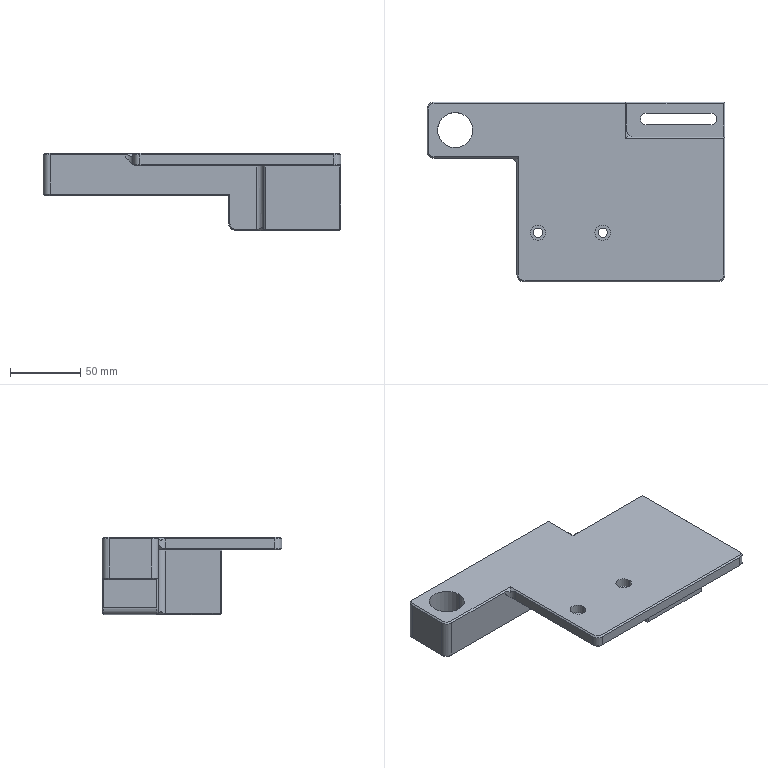NC program | NX | posted with a generic post | part box 212 x 128 x 55 mm
Lines 6898 to 8014 of 8014:
(ZLEVEL_PROFILE_1_COPY , TOOL : D6)
N13746 T07 M6
N13748 G54
N13750 G17 G0 G90 X-54.017 Y50.9 S4000 M3
N13752 G43 Z30. H7
N13754 Z-4.5
N13756 G94 G1 X-49.741 Z-4.724 F1000.
N13758 X-49.265 Y51.142 Z-4.752
N13760 X-48.96 Y51.559 Z-4.779
N13762 X-48.888 Y52.201 Z-4.813
N13764 X-49.179 Y52.777 Z-4.847
N13766 X-49.611 Y53.061 Z-4.874
N13768 X-49.741 Y53.1 Z-4.881
N13770 X-73. Z-6.1
N13772 X-96. F1400.
N13774 G3 X-97.1 Y52. R1.1
N13776 X-96. Y50.9 R1.1
N13778 G1 X-50.
N13780 G3 X-48.9 Y52. R1.1
N13782 X-50. Y53.1 R1.1
N13784 G1 X-73.
N13786 X-78.729 Z-6.2
N13788 X-96.
N13790 G3 X-97.1 Y52. R1.1
N13792 X-96. Y50.9 R1.1
N13794 G1 X-50.
N13796 G3 X-48.9 Y52. R1.1
N13798 X-50. Y53.1 R1.1
N13800 G1 X-73.
N13802 X-78.729 Z-6.3
N13804 X-96.
N13806 G3 X-97.1 Y52. R1.1
N13808 X-96. Y50.9 R1.1
N13810 G1 X-50.
N13812 G3 X-48.9 Y52. R1.1
N13814 X-50. Y53.1 R1.1
N13816 G1 X-73.
N13818 X-78.729 Z-6.4
N13820 X-96.
N13822 G3 X-97.1 Y52. R1.1
N13824 X-96. Y50.9 R1.1
N13826 G1 X-50.
N13828 G3 X-48.9 Y52. R1.1
N13830 X-50. Y53.1 R1.1
N13832 G1 X-73.
N13834 X-78.729 Z-6.5
N13836 X-96.
N13838 G3 X-97.1 Y52. R1.1
N13840 X-96. Y50.9 R1.1
N13842 G1 X-50.
N13844 G3 X-48.9 Y52. R1.1
N13846 X-50. Y53.1 R1.1
N13848 G1 X-73.
N13850 X-78.729 Z-6.6
N13852 X-96.
N13854 G3 X-97.1 Y52. R1.1
N13856 X-96. Y50.9 R1.1
N13858 G1 X-50.
N13860 G3 X-48.9 Y52. R1.1
N13862 X-50. Y53.1 R1.1
N13864 G1 X-73.
N13866 X-78.729 Z-6.7
N13868 X-96.
N13870 G3 X-97.1 Y52. R1.1
N13872 X-96. Y50.9 R1.1
N13874 G1 X-50.
N13876 G3 X-48.9 Y52. R1.1
N13878 X-50. Y53.1 R1.1
N13880 G1 X-73.
N13882 X-78.729 Z-6.8
N13884 X-96.
N13886 G3 X-97.1 Y52. R1.1
N13888 X-96. Y50.9 R1.1
N13890 G1 X-50.
N13892 G3 X-48.9 Y52. R1.1
N13894 X-50. Y53.1 R1.1
N13896 G1 X-73.
N13898 X-78.729 Z-6.9
N13900 X-96.
N13902 G3 X-97.1 Y52. R1.1
N13904 X-96. Y50.9 R1.1
N13906 G1 X-50.
N13908 G3 X-48.9 Y52. R1.1
N13910 X-50. Y53.1 R1.1
N13912 G1 X-73.
N13914 X-78.729 Z-7.
N13916 X-96.
N13918 G3 X-97.1 Y52. R1.1
N13920 X-96. Y50.9 R1.1
N13922 G1 X-50.
N13924 G3 X-48.9 Y52. R1.1
N13926 X-50. Y53.1 R1.1
N13928 G1 X-73.
N13930 X-78.729 Z-7.1
N13932 X-96.
N13934 G3 X-97.1 Y52. R1.1
N13936 X-96. Y50.9 R1.1
N13938 G1 X-50.
N13940 G3 X-48.9 Y52. R1.1
N13942 X-50. Y53.1 R1.1
N13944 G1 X-73.
N13946 X-78.729 Z-7.2
N13948 X-96.
N13950 G3 X-97.1 Y52. R1.1
N13952 X-96. Y50.9 R1.1
N13954 G1 X-50.
N13956 G3 X-48.9 Y52. R1.1
N13958 X-50. Y53.1 R1.1
N13960 G1 X-73.
N13962 X-78.729 Z-7.3
N13964 X-96.
N13966 G3 X-97.1 Y52. R1.1
N13968 X-96. Y50.9 R1.1
N13970 G1 X-50.
N13972 G3 X-48.9 Y52. R1.1
N13974 X-50. Y53.1 R1.1
N13976 G1 X-73.
N13978 X-78.729 Z-7.4
N13980 X-96.
N13982 G3 X-97.1 Y52. R1.1
N13984 X-96. Y50.9 R1.1
N13986 G1 X-50.
N13988 G3 X-48.9 Y52. R1.1
N13990 X-50. Y53.1 R1.1
N13992 G1 X-73.
N13994 X-78.729 Z-7.5
N13996 X-96.
N13998 G3 X-97.1 Y52. R1.1
N14000 X-96. Y50.9 R1.1
N14002 G1 X-50.
N14004 G3 X-48.9 Y52. R1.1
N14006 X-50. Y53.1 R1.1
N14008 G1 X-73.
N14010 X-78.729 Z-7.6
N14012 X-96.
N14014 G3 X-97.1 Y52. R1.1
N14016 X-96. Y50.9 R1.1
N14018 G1 X-50.
N14020 G3 X-48.9 Y52. R1.1
N14022 X-50. Y53.1 R1.1
N14024 G1 X-73.
N14026 X-78.729 Z-7.7
N14028 X-96.
N14030 G3 X-97.1 Y52. R1.1
N14032 X-96. Y50.9 R1.1
N14034 G1 X-50.
N14036 G3 X-48.9 Y52. R1.1
N14038 X-50. Y53.1 R1.1
N14040 G1 X-73.
N14042 X-78.729 Z-7.8
N14044 X-96.
N14046 G3 X-97.1 Y52. R1.1
N14048 X-96. Y50.9 R1.1
N14050 G1 X-50.
N14052 G3 X-48.9 Y52. R1.1
N14054 X-50. Y53.1 R1.1
N14056 G1 X-73.
N14058 X-78.729 Z-7.9
N14060 X-96.
N14062 G3 X-97.1 Y52. R1.1
N14064 X-96. Y50.9 R1.1
N14066 G1 X-50.
N14068 G3 X-48.9 Y52. R1.1
N14070 X-50. Y53.1 R1.1
N14072 G1 X-73.
N14074 X-78.729 Z-8.
N14076 X-96.
N14078 G3 X-97.1 Y52. R1.1
N14080 X-96. Y50.9 R1.1
N14082 G1 X-50.
N14084 G3 X-48.9 Y52. R1.1
N14086 X-50. Y53.1 R1.1
N14088 G1 X-73.
N14090 X-78.729 Z-8.1
N14092 X-96.
N14094 G3 X-97.1 Y52. R1.1
N14096 X-96. Y50.9 R1.1
N14098 G1 X-50.
N14100 G3 X-48.9 Y52. R1.1
N14102 X-50. Y53.1 R1.1
N14104 G1 X-73.
N14106 X-78.729 Z-8.2
N14108 X-96.
N14110 G3 X-97.1 Y52. R1.1
N14112 X-96. Y50.9 R1.1
N14114 G1 X-50.
N14116 G3 X-48.9 Y52. R1.1
N14118 X-50. Y53.1 R1.1
N14120 G1 X-73.
N14122 X-78.729 Z-8.3
N14124 X-96.
N14126 G3 X-97.1 Y52. R1.1
N14128 X-96. Y50.9 R1.1
N14130 G1 X-50.
N14132 G3 X-48.9 Y52. R1.1
N14134 X-50. Y53.1 R1.1
N14136 G1 X-73.
N14138 X-78.729 Z-8.4
N14140 X-96.
N14142 G3 X-97.1 Y52. R1.1
N14144 X-96. Y50.9 R1.1
N14146 G1 X-50.
N14148 G3 X-48.9 Y52. R1.1
N14150 X-50. Y53.1 R1.1
N14152 G1 X-73.
N14154 X-78.729 Z-8.5
N14156 X-96.
N14158 G3 X-97.1 Y52. R1.1
N14160 X-96. Y50.9 R1.1
N14162 G1 X-50.
N14164 G3 X-48.9 Y52. R1.1
N14166 X-50. Y53.1 R1.1
N14168 G1 X-73.
N14170 X-78.729 Z-8.6
N14172 X-96.
N14174 G3 X-97.1 Y52. R1.1
N14176 X-96. Y50.9 R1.1
N14178 G1 X-50.
N14180 G3 X-48.9 Y52. R1.1
N14182 X-50. Y53.1 R1.1
N14184 G1 X-73.
N14186 X-78.729 Z-8.7
N14188 X-96.
N14190 G3 X-97.1 Y52. R1.1
N14192 X-96. Y50.9 R1.1
N14194 G1 X-50.
N14196 G3 X-48.9 Y52. R1.1
N14198 X-50. Y53.1 R1.1
N14200 G1 X-73.
N14202 X-78.729 Z-8.8
N14204 X-96.
N14206 G3 X-97.1 Y52. R1.1
N14208 X-96. Y50.9 R1.1
N14210 G1 X-50.
N14212 G3 X-48.9 Y52. R1.1
N14214 X-50. Y53.1 R1.1
N14216 G1 X-73.
N14218 X-78.729 Z-8.9
N14220 X-96.
N14222 G3 X-97.1 Y52. R1.1
N14224 X-96. Y50.9 R1.1
N14226 G1 X-50.
N14228 G3 X-48.9 Y52. R1.1
N14230 X-50. Y53.1 R1.1
N14232 G1 X-73.
N14234 X-78.729 Z-9.
N14236 X-96.
N14238 G3 X-97.1 Y52. R1.1
N14240 X-96. Y50.9 R1.1
N14242 G1 X-50.
N14244 G3 X-48.9 Y52. R1.1
N14246 X-50. Y53.1 R1.1
N14248 G1 X-73.
N14250 X-78.729 Z-9.1
N14252 X-96.
N14254 G3 X-97.1 Y52. R1.1
N14256 X-96. Y50.9 R1.1
N14258 G1 X-50.
N14260 G3 X-48.9 Y52. R1.1
N14262 X-50. Y53.1 R1.1
N14264 G1 X-73.
N14266 X-78.729 Z-9.2
N14268 X-96.
N14270 G3 X-97.1 Y52. R1.1
N14272 X-96. Y50.9 R1.1
N14274 G1 X-50.
N14276 G3 X-48.9 Y52. R1.1
N14278 X-50. Y53.1 R1.1
N14280 G1 X-73.
N14282 X-78.729 Z-9.3
N14284 X-96.
N14286 G3 X-97.1 Y52. R1.1
N14288 X-96. Y50.9 R1.1
N14290 G1 X-50.
N14292 G3 X-48.9 Y52. R1.1
N14294 X-50. Y53.1 R1.1
N14296 G1 X-73.
N14298 X-78.729 Z-9.4
N14300 X-96.
N14302 G3 X-97.1 Y52. R1.1
N14304 X-96. Y50.9 R1.1
N14306 G1 X-50.
N14308 G3 X-48.9 Y52. R1.1
N14310 X-50. Y53.1 R1.1
N14312 G1 X-73.
N14314 X-78.729 Z-9.5
N14316 X-96.
N14318 G3 X-97.1 Y52. R1.1
N14320 X-96. Y50.9 R1.1
N14322 G1 X-50.
N14324 G3 X-48.9 Y52. R1.1
N14326 X-50. Y53.1 R1.1
N14328 G1 X-73.
N14330 X-78.729 Z-9.6
N14332 X-96.
N14334 G3 X-97.1 Y52. R1.1
N14336 X-96. Y50.9 R1.1
N14338 G1 X-50.
N14340 G3 X-48.9 Y52. R1.1
N14342 X-50. Y53.1 R1.1
N14344 G1 X-73.
N14346 X-78.729 Z-9.7
N14348 X-96.
N14350 G3 X-97.1 Y52. R1.1
N14352 X-96. Y50.9 R1.1
N14354 G1 X-50.
N14356 G3 X-48.9 Y52. R1.1
N14358 X-50. Y53.1 R1.1
N14360 G1 X-73.
N14362 X-78.729 Z-9.8
N14364 X-96.
N14366 G3 X-97.1 Y52. R1.1
N14368 X-96. Y50.9 R1.1
N14370 G1 X-50.
N14372 G3 X-48.9 Y52. R1.1
N14374 X-50. Y53.1 R1.1
N14376 G1 X-73.
N14378 X-78.729 Z-9.9
N14380 X-96.
N14382 G3 X-97.1 Y52. R1.1
N14384 X-96. Y50.9 R1.1
N14386 G1 X-50.
N14388 G3 X-48.9 Y52. R1.1
N14390 X-50. Y53.1 R1.1
N14392 G1 X-73.
N14394 X-78.729 Z-10.
N14396 X-96.
N14398 G3 X-97.1 Y52. R1.1
N14400 X-96. Y50.9 R1.1
N14402 G1 X-50.
N14404 G3 X-48.9 Y52. R1.1
N14406 X-50. Y53.1 R1.1
N14408 G1 X-73.
N14410 X-78.729 Z-10.1
N14412 X-96.
N14414 G3 X-97.1 Y52. R1.1
N14416 X-96. Y50.9 R1.1
N14418 G1 X-50.
N14420 G3 X-48.9 Y52. R1.1
N14422 X-50. Y53.1 R1.1
N14424 G1 X-73.
N14426 X-78.729 Z-10.2
N14428 X-96.
N14430 G3 X-97.1 Y52. R1.1
N14432 X-96. Y50.9 R1.1
N14434 G1 X-50.
N14436 G3 X-48.9 Y52. R1.1
N14438 X-50. Y53.1 R1.1
N14440 G1 X-73.
N14442 X-78.729 Z-10.3
N14444 X-96.
N14446 G3 X-97.1 Y52. R1.1
N14448 X-96. Y50.9 R1.1
N14450 G1 X-50.
N14452 G3 X-48.9 Y52. R1.1
N14454 X-50. Y53.1 R1.1
N14456 G1 X-73.
N14458 X-78.729 Z-10.4
N14460 X-96.
N14462 G3 X-97.1 Y52. R1.1
N14464 X-96. Y50.9 R1.1
N14466 G1 X-50.
N14468 G3 X-48.9 Y52. R1.1
N14470 X-50. Y53.1 R1.1
N14472 G1 X-73.
N14474 X-78.729 Z-10.5
N14476 X-96.
N14478 G3 X-97.1 Y52. R1.1
N14480 X-96. Y50.9 R1.1
N14482 G1 X-50.
N14484 G3 X-48.9 Y52. R1.1
N14486 X-50. Y53.1 R1.1
N14488 G1 X-73.
N14490 X-78.729 Z-10.6
N14492 X-96.
N14494 G3 X-97.1 Y52. R1.1
N14496 X-96. Y50.9 R1.1
N14498 G1 X-50.
N14500 G3 X-48.9 Y52. R1.1
N14502 X-50. Y53.1 R1.1
N14504 G1 X-73.
N14506 X-78.729 Z-10.7
N14508 X-96.
N14510 G3 X-97.1 Y52. R1.1
N14512 X-96. Y50.9 R1.1
N14514 G1 X-50.
N14516 G3 X-48.9 Y52. R1.1
N14518 X-50. Y53.1 R1.1
N14520 G1 X-73.
N14522 X-78.729 Z-10.8
N14524 X-96.
N14526 G3 X-97.1 Y52. R1.1
N14528 X-96. Y50.9 R1.1
N14530 G1 X-50.
N14532 G3 X-48.9 Y52. R1.1
N14534 X-50. Y53.1 R1.1
N14536 G1 X-73.
N14538 X-78.729 Z-10.9
N14540 X-96.
N14542 G3 X-97.1 Y52. R1.1
N14544 X-96. Y50.9 R1.1
N14546 G1 X-50.
N14548 G3 X-48.9 Y52. R1.1
N14550 X-50. Y53.1 R1.1
N14552 G1 X-73.
N14554 X-78.729 Z-11.
N14556 X-96.
N14558 G3 X-97.1 Y52. R1.1
N14560 X-96. Y50.9 R1.1
N14562 G1 X-50.
N14564 G3 X-48.9 Y52. R1.1
N14566 X-50. Y53.1 R1.1
N14568 G1 X-73.
N14570 X-78.729 Z-11.1
N14572 X-96.
N14574 G3 X-97.1 Y52. R1.1
N14576 X-96. Y50.9 R1.1
N14578 G1 X-50.
N14580 G3 X-48.9 Y52. R1.1
N14582 X-50. Y53.1 R1.1
N14584 G1 X-73.
N14586 X-78.729 Z-11.2
N14588 X-96.
N14590 G3 X-97.1 Y52. R1.1
N14592 X-96. Y50.9 R1.1
N14594 G1 X-50.
N14596 G3 X-48.9 Y52. R1.1
N14598 X-50. Y53.1 R1.1
N14600 G1 X-73.
N14602 X-78.729 Z-11.3
N14604 X-96.
N14606 G3 X-97.1 Y52. R1.1
N14608 X-96. Y50.9 R1.1
N14610 G1 X-50.
N14612 G3 X-48.9 Y52. R1.1
N14614 X-50. Y53.1 R1.1
N14616 G1 X-73.
N14618 X-78.729 Z-11.4
N14620 X-96.
N14622 G3 X-97.1 Y52. R1.1
N14624 X-96. Y50.9 R1.1
N14626 G1 X-50.
N14628 G3 X-48.9 Y52. R1.1
N14630 X-50. Y53.1 R1.1
N14632 G1 X-73.
N14634 X-78.729 Z-11.5
N14636 X-96.
N14638 G3 X-97.1 Y52. R1.1
N14640 X-96. Y50.9 R1.1
N14642 G1 X-50.
N14644 G3 X-48.9 Y52. R1.1
N14646 X-50. Y53.1 R1.1
N14648 G1 X-73.
N14650 X-78.729 Z-11.6
N14652 X-96.
N14654 G3 X-97.1 Y52. R1.1
N14656 X-96. Y50.9 R1.1
N14658 G1 X-50.
N14660 G3 X-48.9 Y52. R1.1
N14662 X-50. Y53.1 R1.1
N14664 G1 X-73.
N14666 X-78.729 Z-11.7
N14668 X-96.
N14670 G3 X-97.1 Y52. R1.1
N14672 X-96. Y50.9 R1.1
N14674 G1 X-50.
N14676 G3 X-48.9 Y52. R1.1
N14678 X-50. Y53.1 R1.1
N14680 G1 X-73.
N14682 X-78.729 Z-11.8
N14684 X-96.
N14686 G3 X-97.1 Y52. R1.1
N14688 X-96. Y50.9 R1.1
N14690 G1 X-50.
N14692 G3 X-48.9 Y52. R1.1
N14694 X-50. Y53.1 R1.1
N14696 G1 X-73.
N14698 X-78.729 Z-11.9
N14700 X-96.
N14702 G3 X-97.1 Y52. R1.1
N14704 X-96. Y50.9 R1.1
N14706 G1 X-50.
N14708 G3 X-48.9 Y52. R1.1
N14710 X-50. Y53.1 R1.1
N14712 G1 X-73.
N14714 X-78.729 Z-12.
N14716 X-96.
N14718 G3 X-97.1 Y52. R1.1
N14720 X-96. Y50.9 R1.1
N14722 G1 X-50.
N14724 G3 X-48.9 Y52. R1.1
N14726 X-50. Y53.1 R1.1
N14728 G1 X-73.
N14730 X-78.729 Z-12.1
N14732 X-96.
N14734 G3 X-97.1 Y52. R1.1
N14736 X-96. Y50.9 R1.1
N14738 G1 X-50.
N14740 G3 X-48.9 Y52. R1.1
N14742 X-50. Y53.1 R1.1
N14744 G1 X-73.
N14746 X-78.729 Z-12.2
N14748 X-96.
N14750 G3 X-97.1 Y52. R1.1
N14752 X-96. Y50.9 R1.1
N14754 G1 X-50.
N14756 G3 X-48.9 Y52. R1.1
N14758 X-50. Y53.1 R1.1
N14760 G1 X-73.
N14762 X-78.729 Z-12.3
N14764 X-96.
N14766 G3 X-97.1 Y52. R1.1
N14768 X-96. Y50.9 R1.1
N14770 G1 X-50.
N14772 G3 X-48.9 Y52. R1.1
N14774 X-50. Y53.1 R1.1
N14776 G1 X-73.
N14778 X-78.729 Z-12.4
N14780 X-96.
N14782 G3 X-97.1 Y52. R1.1
N14784 X-96. Y50.9 R1.1
N14786 G1 X-50.
N14788 G3 X-48.9 Y52. R1.1
N14790 X-50. Y53.1 R1.1
N14792 G1 X-73.
N14794 X-78.729 Z-12.5
N14796 X-96.
N14798 G3 X-97.1 Y52. R1.1
N14800 X-96. Y50.9 R1.1
N14802 G1 X-50.
N14804 G3 X-48.9 Y52. R1.1
N14806 X-50. Y53.1 R1.1
N14808 G1 X-73.
N14810 X-78.729 Z-12.6
N14812 X-96.
N14814 G3 X-97.1 Y52. R1.1
N14816 X-96. Y50.9 R1.1
N14818 G1 X-50.
N14820 G3 X-48.9 Y52. R1.1
N14822 X-50. Y53.1 R1.1
N14824 G1 X-73.
N14826 X-78.729 Z-12.7
N14828 X-96.
N14830 G3 X-97.1 Y52. R1.1
N14832 X-96. Y50.9 R1.1
N14834 G1 X-50.
N14836 G3 X-48.9 Y52. R1.1
N14838 X-50. Y53.1 R1.1
N14840 G1 X-73.
N14842 X-78.729 Z-12.8
N14844 X-96.
N14846 G3 X-97.1 Y52. R1.1
N14848 X-96. Y50.9 R1.1
N14850 G1 X-50.
N14852 G3 X-48.9 Y52. R1.1
N14854 X-50. Y53.1 R1.1
N14856 G1 X-73.
N14858 X-78.729 Z-12.9
N14860 X-96.
N14862 G3 X-97.1 Y52. R1.1
N14864 X-96. Y50.9 R1.1
N14866 G1 X-50.
N14868 G3 X-48.9 Y52. R1.1
N14870 X-50. Y53.1 R1.1
N14872 G1 X-73.
N14874 X-78.729 Z-13.
N14876 X-96.
N14878 G3 X-97.1 Y52. R1.1
N14880 X-96. Y50.9 R1.1
N14882 G1 X-50.
N14884 G3 X-48.9 Y52. R1.1
N14886 X-50. Y53.1 R1.1
N14888 G1 X-73.
N14890 X-78.729 Z-13.1
N14892 X-96.
N14894 G3 X-97.1 Y52. R1.1
N14896 X-96. Y50.9 R1.1
N14898 G1 X-50.
N14900 G3 X-48.9 Y52. R1.1
N14902 X-50. Y53.1 R1.1
N14904 G1 X-73.
N14906 X-78.729 Z-13.2
N14908 X-96.
N14910 G3 X-97.1 Y52. R1.1
N14912 X-96. Y50.9 R1.1
N14914 G1 X-50.
N14916 G3 X-48.9 Y52. R1.1
N14918 X-50. Y53.1 R1.1
N14920 G1 X-73.
N14922 X-78.729 Z-13.3
N14924 X-96.
N14926 G3 X-97.1 Y52. R1.1
N14928 X-96. Y50.9 R1.1
N14930 G1 X-50.
N14932 G3 X-48.9 Y52. R1.1
N14934 X-50. Y53.1 R1.1
N14936 G1 X-73.
N14938 X-78.729 Z-13.4
N14940 X-96.
N14942 G3 X-97.1 Y52. R1.1
N14944 X-96. Y50.9 R1.1
N14946 G1 X-50.
N14948 G3 X-48.9 Y52. R1.1
N14950 X-50. Y53.1 R1.1
N14952 G1 X-73.
N14954 X-78.729 Z-13.5
N14956 X-96.
N14958 G3 X-97.1 Y52. R1.1
N14960 X-96. Y50.9 R1.1
N14962 G1 X-50.
N14964 G3 X-48.9 Y52. R1.1
N14966 X-50. Y53.1 R1.1
N14968 G1 X-73.
N14970 X-78.729 Z-13.6
N14972 X-96.
N14974 G3 X-97.1 Y52. R1.1
N14976 X-96. Y50.9 R1.1
N14978 G1 X-50.
N14980 G3 X-48.9 Y52. R1.1
N14982 X-50. Y53.1 R1.1
N14984 G1 X-73.
N14986 X-78.729 Z-13.7
N14988 X-96.
N14990 G3 X-97.1 Y52. R1.1
N14992 X-96. Y50.9 R1.1
N14994 G1 X-50.
N14996 G3 X-48.9 Y52. R1.1
N14998 X-50. Y53.1 R1.1
N15000 G1 X-73.
N15002 X-78.729 Z-13.8
N15004 X-96.
N15006 G3 X-97.1 Y52. R1.1
N15008 X-96. Y50.9 R1.1
N15010 G1 X-50.
N15012 G3 X-48.9 Y52. R1.1
N15014 X-50. Y53.1 R1.1
N15016 G1 X-73.
N15018 X-78.729 Z-13.9
N15020 X-96.
N15022 G3 X-97.1 Y52. R1.1
N15024 X-96. Y50.9 R1.1
N15026 G1 X-50.
N15028 G3 X-48.9 Y52. R1.1
N15030 X-50. Y53.1 R1.1
N15032 G1 X-73.
N15034 X-78.729 Z-14.
N15036 X-96.
N15038 G3 X-97.1 Y52. R1.1
N15040 X-96. Y50.9 R1.1
N15042 G1 X-50.
N15044 G3 X-48.9 Y52. R1.1
N15046 X-50. Y53.1 R1.1
N15048 G1 X-73.
N15050 X-78.729 Z-14.1
N15052 X-96.
N15054 G3 X-97.1 Y52. R1.1
N15056 X-96. Y50.9 R1.1
N15058 G1 X-50.
N15060 G3 X-48.9 Y52. R1.1
N15062 X-50. Y53.1 R1.1
N15064 G1 X-73.
N15066 X-78.729 Z-14.2
N15068 X-96.
N15070 G3 X-97.1 Y52. R1.1
N15072 X-96. Y50.9 R1.1
N15074 G1 X-50.
N15076 G3 X-48.9 Y52. R1.1
N15078 X-50. Y53.1 R1.1
N15080 G1 X-73.
N15082 X-78.729 Z-14.3
N15084 X-96.
N15086 G3 X-97.1 Y52. R1.1
N15088 X-96. Y50.9 R1.1
N15090 G1 X-50.
N15092 G3 X-48.9 Y52. R1.1
N15094 X-50. Y53.1 R1.1
N15096 G1 X-73.
N15098 X-78.729 Z-14.4
N15100 X-96.
N15102 G3 X-97.1 Y52. R1.1
N15104 X-96. Y50.9 R1.1
N15106 G1 X-50.
N15108 G3 X-48.9 Y52. R1.1
N15110 X-50. Y53.1 R1.1
N15112 G1 X-73.
N15114 X-78.729 Z-14.5
N15116 X-96.
N15118 G3 X-97.1 Y52. R1.1
N15120 X-96. Y50.9 R1.1
N15122 G1 X-50.
N15124 G3 X-48.9 Y52. R1.1
N15126 X-50. Y53.1 R1.1
N15128 G1 X-73.
N15130 X-78.729 Z-14.6
N15132 X-96.
N15134 G3 X-97.1 Y52. R1.1
N15136 X-96. Y50.9 R1.1
N15138 G1 X-50.
N15140 G3 X-48.9 Y52. R1.1
N15142 X-50. Y53.1 R1.1
N15144 G1 X-73.
N15146 X-78.729 Z-14.7
N15148 X-96.
N15150 G3 X-97.1 Y52. R1.1
N15152 X-96. Y50.9 R1.1
N15154 G1 X-50.
N15156 G3 X-48.9 Y52. R1.1
N15158 X-50. Y53.1 R1.1
N15160 G1 X-73.
N15162 X-78.729 Z-14.8
N15164 X-96.
N15166 G3 X-97.1 Y52. R1.1
N15168 X-96. Y50.9 R1.1
N15170 G1 X-50.
N15172 G3 X-48.9 Y52. R1.1
N15174 X-50. Y53.1 R1.1
N15176 G1 X-73.
N15178 X-78.729 Z-14.9
N15180 X-96.
N15182 G3 X-97.1 Y52. R1.1
N15184 X-96. Y50.9 R1.1
N15186 G1 X-50.
N15188 G3 X-48.9 Y52. R1.1
N15190 X-50. Y53.1 R1.1
N15192 G1 X-73.
N15194 X-78.729 Z-15.
N15196 X-96.
N15198 G3 X-97.1 Y52. R1.1
N15200 X-96. Y50.9 R1.1
N15202 G1 X-50.
N15204 G3 X-48.9 Y52. R1.1
N15206 X-50. Y53.1 R1.1
N15208 G1 X-73.
N15210 X-78.729 Z-15.1
N15212 X-96.
N15214 G3 X-97.1 Y52. R1.1
N15216 X-96. Y50.9 R1.1
N15218 G1 X-50.
N15220 G3 X-48.9 Y52. R1.1
N15222 X-50. Y53.1 R1.1
N15224 G1 X-73.
N15226 X-78.729 Z-15.2
N15228 X-96.
N15230 G3 X-97.1 Y52. R1.1
N15232 X-96. Y50.9 R1.1
N15234 G1 X-50.
N15236 G3 X-48.9 Y52. R1.1
N15238 X-50. Y53.1 R1.1
N15240 G1 X-73.
N15242 X-78.729 Z-15.3
N15244 X-96.
N15246 G3 X-97.1 Y52. R1.1
N15248 X-96. Y50.9 R1.1
N15250 G1 X-50.
N15252 G3 X-48.9 Y52. R1.1
N15254 X-50. Y53.1 R1.1
N15256 G1 X-73.
N15258 X-78.729 Z-15.4
N15260 X-96.
N15262 G3 X-97.1 Y52. R1.1
N15264 X-96. Y50.9 R1.1
N15266 G1 X-50.
N15268 G3 X-48.9 Y52. R1.1
N15270 X-50. Y53.1 R1.1
N15272 G1 X-73.
N15274 X-78.729 Z-15.5
N15276 X-96.
N15278 G3 X-97.1 Y52. R1.1
N15280 X-96. Y50.9 R1.1
N15282 G1 X-50.
N15284 G3 X-48.9 Y52. R1.1
N15286 X-50. Y53.1 R1.1
N15288 G1 X-73.
N15290 X-78.729 Z-15.6
N15292 X-96.
N15294 G3 X-97.1 Y52. R1.1
N15296 X-96. Y50.9 R1.1
N15298 G1 X-50.
N15300 G3 X-48.9 Y52. R1.1
N15302 X-50. Y53.1 R1.1
N15304 G1 X-73.
N15306 X-78.729 Z-15.7
N15308 X-96.
N15310 G3 X-97.1 Y52. R1.1
N15312 X-96. Y50.9 R1.1
N15314 G1 X-50.
N15316 G3 X-48.9 Y52. R1.1
N15318 X-50. Y53.1 R1.1
N15320 G1 X-73.
N15322 X-78.729 Z-15.8
N15324 X-96.
N15326 G3 X-97.1 Y52. R1.1
N15328 X-96. Y50.9 R1.1
N15330 G1 X-50.
N15332 G3 X-48.9 Y52. R1.1
N15334 X-50. Y53.1 R1.1
N15336 G1 X-73.
N15338 X-78.729 Z-15.9
N15340 X-96.
N15342 G3 X-97.1 Y52. R1.1
N15344 X-96. Y50.9 R1.1
N15346 G1 X-50.
N15348 G3 X-48.9 Y52. R1.1
N15350 X-50. Y53.1 R1.1
N15352 G1 X-73.
N15354 X-78.729 Z-16.
N15356 X-96.
N15358 G3 X-97.1 Y52. R1.1
N15360 X-96. Y50.9 R1.1
N15362 G1 X-50.
N15364 G3 X-48.9 Y52. R1.1
N15366 X-50. Y53.1 R1.1
N15368 G1 X-73.
N15370 X-78.729 Z-16.1
N15372 X-96.
N15374 G3 X-97.1 Y52. R1.1
N15376 X-96. Y50.9 R1.1
N15378 G1 X-50.
N15380 G3 X-48.9 Y52. R1.1
N15382 X-50. Y53.1 R1.1
N15384 G1 X-73.
N15386 X-78.729 Z-16.2
N15388 X-96.
N15390 G3 X-97.1 Y52. R1.1
N15392 X-96. Y50.9 R1.1
N15394 G1 X-50.
N15396 G3 X-48.9 Y52. R1.1
N15398 X-50. Y53.1 R1.1
N15400 G1 X-73.
N15402 X-78.729 Z-16.3
N15404 X-96.
N15406 G3 X-97.1 Y52. R1.1
N15408 X-96. Y50.9 R1.1
N15410 G1 X-50.
N15412 G3 X-48.9 Y52. R1.1
N15414 X-50. Y53.1 R1.1
N15416 G1 X-73.
N15418 X-78.729 Z-16.4
N15420 X-96.
N15422 G3 X-97.1 Y52. R1.1
N15424 X-96. Y50.9 R1.1
N15426 G1 X-50.
N15428 G3 X-48.9 Y52. R1.1
N15430 X-50. Y53.1 R1.1
N15432 G1 X-73.
N15434 X-78.729 Z-16.5
N15436 X-96.
N15438 G3 X-97.1 Y52. R1.1
N15440 X-96. Y50.9 R1.1
N15442 G1 X-50.
N15444 G3 X-48.9 Y52. R1.1
N15446 X-50. Y53.1 R1.1
N15448 G1 X-73.
N15450 X-78.729 Z-16.6
N15452 X-96.
N15454 G3 X-97.1 Y52. R1.1
N15456 X-96. Y50.9 R1.1
N15458 G1 X-50.
N15460 G3 X-48.9 Y52. R1.1
N15462 X-50. Y53.1 R1.1
N15464 G1 X-73.
N15466 X-78.729 Z-16.7
N15468 X-96.
N15470 G3 X-97.1 Y52. R1.1
N15472 X-96. Y50.9 R1.1
N15474 G1 X-50.
N15476 G3 X-48.9 Y52. R1.1
N15478 X-50. Y53.1 R1.1
N15480 G1 X-73.
N15482 X-78.729 Z-16.8
N15484 X-96.
N15486 G3 X-97.1 Y52. R1.1
N15488 X-96. Y50.9 R1.1
N15490 G1 X-50.
N15492 G3 X-48.9 Y52. R1.1
N15494 X-50. Y53.1 R1.1
N15496 G1 X-73.
N15498 X-78.729 Z-16.9
N15500 X-96.
N15502 G3 X-97.1 Y52. R1.1
N15504 X-96. Y50.9 R1.1
N15506 G1 X-50.
N15508 G3 X-48.9 Y52. R1.1
N15510 X-50. Y53.1 R1.1
N15512 G1 X-73.
N15514 X-78.729 Z-17.
N15516 X-96.
N15518 G3 X-97.1 Y52. R1.1
N15520 X-96. Y50.9 R1.1
N15522 G1 X-50.
N15524 G3 X-48.9 Y52. R1.1
N15526 X-50. Y53.1 R1.1
N15528 G1 X-73.
N15530 X-78.729 Z-17.1
N15532 X-96.
N15534 G3 X-97.1 Y52. R1.1
N15536 X-96. Y50.9 R1.1
N15538 G1 X-50.
N15540 G3 X-48.9 Y52. R1.1
N15542 X-50. Y53.1 R1.1
N15544 G1 X-73.
N15546 X-78.729 Z-17.2
N15548 X-96.
N15550 G3 X-97.1 Y52. R1.1
N15552 X-96. Y50.9 R1.1
N15554 G1 X-50.
N15556 G3 X-48.9 Y52. R1.1
N15558 X-50. Y53.1 R1.1
N15560 G1 X-73.
N15562 X-78.729 Z-17.3
N15564 X-96.
N15566 G3 X-97.1 Y52. R1.1
N15568 X-96. Y50.9 R1.1
N15570 G1 X-50.
N15572 G3 X-48.9 Y52. R1.1
N15574 X-50. Y53.1 R1.1
N15576 G1 X-73.
N15578 X-78.729 Z-17.4
N15580 X-96.
N15582 G3 X-97.1 Y52. R1.1
N15584 X-96. Y50.9 R1.1
N15586 G1 X-50.
N15588 G3 X-48.9 Y52. R1.1
N15590 X-50. Y53.1 R1.1
N15592 G1 X-73.
N15594 X-78.729 Z-17.5
N15596 X-96.
N15598 G3 X-97.1 Y52. R1.1
N15600 X-96. Y50.9 R1.1
N15602 G1 X-50.
N15604 G3 X-48.9 Y52. R1.1
N15606 X-50. Y53.1 R1.1
N15608 G1 X-73.
N15610 X-78.729 Z-17.6
N15612 X-96.
N15614 G3 X-97.1 Y52. R1.1
N15616 X-96. Y50.9 R1.1
N15618 G1 X-50.
N15620 G3 X-48.9 Y52. R1.1
N15622 X-50. Y53.1 R1.1
N15624 G1 X-73.
N15626 X-78.729 Z-17.7
N15628 X-96.
N15630 G3 X-97.1 Y52. R1.1
N15632 X-96. Y50.9 R1.1
N15634 G1 X-50.
N15636 G3 X-48.9 Y52. R1.1
N15638 X-50. Y53.1 R1.1
N15640 G1 X-73.
N15642 X-78.729 Z-17.8
N15644 X-96.
N15646 G3 X-97.1 Y52. R1.1
N15648 X-96. Y50.9 R1.1
N15650 G1 X-50.
N15652 G3 X-48.9 Y52. R1.1
N15654 X-50. Y53.1 R1.1
N15656 G1 X-73.
N15658 X-78.729 Z-17.9
N15660 X-96.
N15662 G3 X-97.1 Y52. R1.1
N15664 X-96. Y50.9 R1.1
N15666 G1 X-50.
N15668 G3 X-48.9 Y52. R1.1
N15670 X-50. Y53.1 R1.1
N15672 G1 X-73.
N15674 X-78.729 Z-18.
N15676 X-96.
N15678 G3 X-97.1 Y52. R1.1
N15680 X-96. Y50.9 R1.1
N15682 G1 X-50.
N15684 G3 X-48.9 Y52. R1.1
N15686 X-50. Y53.1 R1.1
N15688 G1 X-78.729
N15690 Z-16.5
N15692 G0 Z30.
N15694 M5
(ZLEVEL_PROFILE_1_COPY_1_COPY_COPY_1_COPY_COPY_COPY , TOOL : D8A45)
N15696 T06 M6
N15698 G54
N15700 G17 G0 G90 X-31.011 Y20.271 S6500 M3
N15702 G43 Z30. H6
N15704 Z-2.
N15706 G94 G1 Z-3. F1000.
N15708 X-31.308 Y21.428
N15710 G3 X-31.867 Y22. R0.8
N15712 G1 X-48.997
N15714 X-49. Y21.737
N15716 Y-20.499
N15718 G2 X-49.778 Y-22.311 R2.499
N15720 X-51.464 Y-22.994 R2.487
N15722 G1 X-51.999 Y-23.
N15724 X-105.001
N15726 X-105.502 Y-22.998
N15728 G2 X-108. Y-20.492 R2.507
N15730 G1 Y-20.002
N15732 Y63.002
N15734 X-107.998 Y63.516
N15736 G2 X-105.515 Y65.998 R2.493
N15738 G1 X-105.001 Y66.
N15740 X-31.867
N15742 G3 X-31.308 Y66.572 R0.8
N15744 G1 X-31.011 Y67.729
N15746 Z-2.
N15748 G0 Z30.
(ZLEVEL_PROFILE_1_COPY_1_COPY_COPY_1_COPY_COPY_COPY_COPY_1 , TOOL : D8A45)
N15750 X-48.385 Y55.086
N15752 Z-1.
N15754 G1 Z-2.
N15756 X-49.307 Y56.683
N15758 G3 X-50. Y57.083 R0.8
N15760 G1 X-96.
N15762 G3 X-101.083 Y52. R5.083
N15764 X-96. Y46.917 R5.083
N15766 G1 X-50.
N15768 G3 X-44.917 Y52. R5.083
N15770 X-50. Y57.083 R5.083
N15772 X-50.693 Y56.683 R0.8
N15774 G1 X-51.386 Y55.483
N15776 Z-1.
N15778 G0 Z30.
(ZLEVEL_PROFILE_1_COPY_1_COPY_COPY_1_COPY_COPY_COPY_COPY , TOOL : D8A45)
N15780 X-21.582 Y66.6
N15782 Z-26.
N15784 G1 Z-27.
N15786 X-22.654 Y65.4
N15788 G3 X-21.962 Y65. R0.8
N15790 G1 X101.
N15792 G2 X107. Y59. R6.
N15794 G1 Y29.
N15796 G2 X101. Y23. R6.
N15798 G1 X-21.962
N15800 G3 X-22.654 Y22.6 R0.8
N15802 G1 X-21.582 Y21.4
N15804 Z-26.
N15806 G0 Z30.
(ZLEVEL_PROFILE_1_COPY_1_COPY_COPY_1_COPY_COPY_COPY_COPY_COPY_1 , TOOL : D8A45)
N15808 X87.454 Y52.864
N15810 Z-26.
N15812 G1 Z-27.
N15814 X86.693 Y54.183
N15816 G3 X86. Y54.583 R0.8
N15818 X75.417 Y44. R10.583
N15820 X86. Y54.583 R-10.583
N15822 X85.307 Y54.183 R0.8
N15824 G1 X84.546 Y52.864
N15826 Z-26.
N15828 G0 Z30.
(ZLEVEL_PROFILE_1_COPY_1_COPY_COPY_1_COPY_COPY_COPY_COPY_COPY , TOOL : D8A45)
N15830 X27. Y-30.3
N15832 Z-45.
N15834 G1 Z-48.
N15836 G3 X28.3 Y-29. R1.3
N15838 X27. Y-30.3 R-1.3
N15840 X27.693 Y-29.9 R0.8
N15842 G1 Z-47.
N15844 G0 Z30.
N15846 X-19. Y-30.3
N15848 Z-45.
N15850 G1 Z-48.
N15852 G3 X-17.7 Y-29. R1.3
N15854 X-19. Y-30.3 R-1.3
N15856 X-18.307 Y-29.9 R0.8
N15858 G1 Z-47.
N15860 G0 Z30.
N15862 X44.6 Y18.4
N15864 Z-47.
N15866 G1 Z-48.
N15868 X43.2 Y19.84
N15870 G3 X43. Y19.493 R0.4
N15872 G1 Y-59.
N15874 G2 X37. Y-65. R6.
N15876 G1 X-101.
N15878 G2 X-107. Y-59. R6.
N15880 G1 Y-25.04
N15882 G3 X-107.4 Y-24.347 R0.8
N15884 G1 X-108.6 Y-25.29
N15886 Z-47.
N15888 G0 Z30.
(ZLEVEL_PROFILE_1_COPY_1_COPY_COPY_1_COPY_COPY_COPY_COPY_COPY_COPY , TOOL : D8A)
N15890 X-19.258 Y-29.739
N15892 Z-46.
N15894 G1 Z-47.
N15896 X-19.693 Y-30.983
N15898 G3 X-19. Y-31.383 R0.8
N15900 X-16.617 Y-29. R2.383
N15902 X-19. Y-31.383 R-2.383
N15904 X-18.307 Y-30.983 R0.8
N15906 G1 X-18.742 Y-29.739
N15908 Z-46.
N15910 G0 Z30.
N15912 X26.742
N15914 Z-46.
N15916 G1 Z-47.
N15918 X26.307 Y-30.983
N15920 G3 X27. Y-31.383 R0.8
N15922 X29.383 Y-29. R2.383
N15924 X27. Y-31.383 R-2.383
N15926 X27.693 Y-30.983 R0.8
N15928 G1 X27.258 Y-29.739
N15930 Z-46.
N15932 G0 Z30.
N15934 M5
N15936 M2